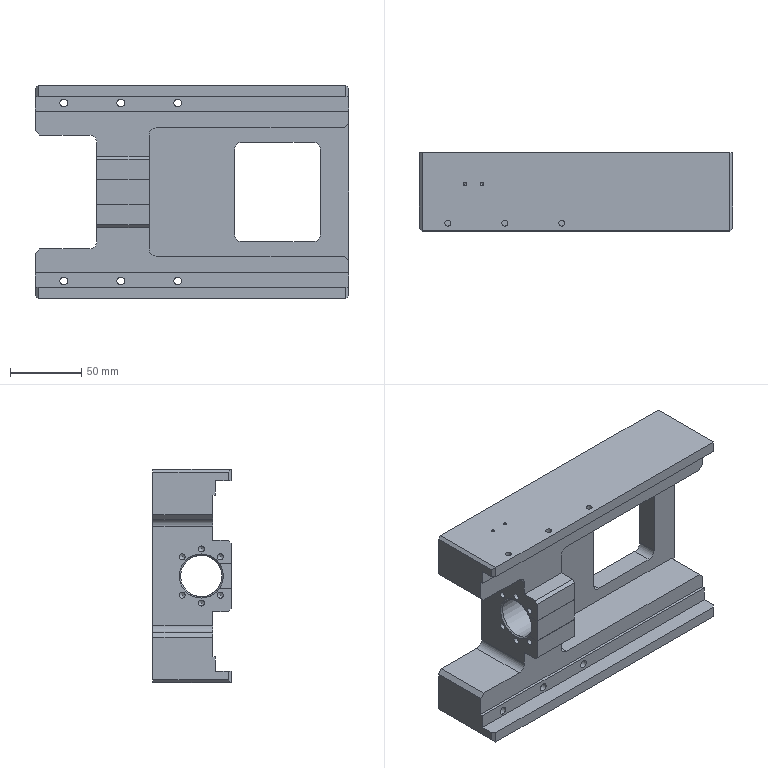CAM job | NX | 3+2 milling, drilling | part box 220 x 55 x 150 mm | stock box 225 x 60 x 155 mm
Tools:
number,name,description,diameter,corner_radius,flute_length,length,flutes
6,D6,平底铣刀-粗,6.0,0.0,25.0,75.0,2
9,D10,平底铣刀-粗,10.0,0.0,35.0,75.0,2
17,D16,平底铣刀-粗,16.0,0.0,50.0,75.0,2
7,D6-J,平底铣刀-精,6.0,0.0,25.0,75.0,2
10,D10-J,平底铣刀-精,10.0,0.0,35.0,75.0,2
18,D16-J,平底铣刀-精,16.0,0.0,50.0,75.0,2
1,D80R0.8飞刀,圆鼻刀-粗,80.0,0.8,50.0,75.0,2
1,D80R0.8飞刀-J,圆鼻刀-精,80.0,0.8,50.0,75.0,2
2,D6倒角刀,倒角刀,6.0,0.0,3.0,25.0,2
19,D10倒角刀,倒角刀,10.0,0.0,5.0,75.0,2
18,M6X1.0,丝锥,5.0,0.0,35.0,50.0,2
15,ZT5,钻头,5.0,0.0,35.0,50.0,2
17,ZT5.5,钻头,5.5,0.0,35.0,50.0,2
14,钻头4.2,Twist Drill 4.2 mm,4.2,0.0,41.0,41.738,2
Operations:
program,operation,operation_type,tool,method,geometry_group,spindle_rpm,surface_speed,feed_per_tooth,feed_cut,feed_plunge,cut_length_mm,path_length_mm,cut_time_min,machine_time_min
C,等高往复层切开粗-中_COPY,ZLevelMilling,D16,分层开粗-切深K-步距G,W-C,5000.0,251.327,0.4,4000.0,100.0,6927.946,7129.946,1.732,1.752
C,打点-深0.8_2,Operation,D10倒角刀,NONE,W-C,5000.0,157.08,0.05,500.0,90.0,10.8,237.794,0.0216,0.0443
C,盲锥孔-M5螺纹底孔,Operation,钻头4.2,NONE,W-C,2500.0,32.987,0.03,150.0,90.0,87.971,392.136,0.5865,0.6169
C,铣倒角_3,PlanarMilling,D10倒角刀,METHOD,W-C,5000.0,157.08,0.05,500.0,100.0,86.111,935.558,0.1722,0.2572
C,底壁铣倒角_COPY_1,VolumeBased25DMillingOperation,D10倒角刀,爬面_倒角-切深0-步距G,W-C,5000.0,157.08,0.05,500.0,100.0,98.589,224.989,0.1972,0.2098
C,C0.3封闭铣廓倒角6X45L_COPY,PlanarMilling,D10倒角刀,爬面_倒角-切深0-步距G,W-C,5000.0,157.08,0.15,1500.0,100.0,41.144,301.88,0.0274,0.0535
C,底壁铣精光侧面-中_COPY,VolumeBased25DMillingOperation,D16-J,侧刃精光-切深K-步距G,W-C,5000.0,251.327,0.1,1000.0,100.0,431.631,640.548,0.4316,0.4525
B,底壁铣飞面开粗_COPY,VolumeBased25DMillingOperation,D80R0.8飞刀,分层开粗-切深K-步距G,W-B,2800.0,703.696,0.5357,3000.0,100.0,8995.189,11896.094,2.998,3.288
B,底壁铣飞面精光_COPY,VolumeBased25DMillingOperation,D80R0.8飞刀-J,侧刃精光-切深K-步距G,W-B,4000.0,1005.28,0.125,1000.0,100.0,998.658,1034.658,0.9987,1.002
B,型腔铣开粗-中_COPY_1,CavityMilling,D10,分层开粗-切深K-步距G,W-B,8000.0,251.327,0.3438,5500.0,100.0,177634.57,185500.312,32.297,33.369
B,底壁铣精光底面-中_COPY,VolumeBased25DMillingOperation,D10-J,精光步距切深关,W-B,7000.0,175.0,0.0536,1500.0,100.0,3210.716,3490.119,2.14,2.168
B,底壁铣精光底面-中_COPY_1,VolumeBased25DMillingOperation,D10-J,精光步距切深关,W-B,7000.0,175.0,0.0536,1500.0,100.0,2341.522,2449.522,1.561,1.572
B,底壁铣精光侧面-中-选底面_COPY_1,VolumeBased25DMillingOperation,D10-J,侧刃精光-切深K-步距G,W-B,8000.0,251.32,0.0625,1000.0,100.0,588.723,828.896,0.5887,0.6127
B,底壁铣精光侧面-中-选底面_COPY_2,VolumeBased25DMillingOperation,D10-J,侧刃精光-切深K-步距G,W-B,8000.0,251.32,0.0625,1000.0,100.0,1114.927,1384.071,1.115,1.142
B,平面去毛刺6X45L_COPY,SurfaceContour,D6倒角刀,爬面_倒角-切深0-步距G,W-B,6500.0,122.519,0.1154,1500.0,100.0,2584.887,4812.187,1.723,1.946
B,底壁铣倒角_COPY,VolumeBased25DMillingOperation,D6倒角刀,爬面_倒角-切深0-步距G,W-B,6500.0,122.519,0.1154,1500.0,100.0,170.429,986.413,0.1136,0.1952
B,底壁铣精光侧面-中-选底面_COPY,VolumeBased25DMillingOperation,D10-J,侧刃精光-切深K-步距G,W-B,8000.0,251.32,0.0625,1000.0,100.0,476.566,671.587,0.4766,0.4961
A,顶面,FaceMilling,D80R0.8飞刀,侧刃精光-切深K-步距G,W-A,4000.0,1005.31,0.125,1000.0,100.0,1352.0,1388.0,1.352,1.356
A,型腔铣开粗-中_COPY,CavityMilling,D10,分层开粗-切深K-步距G,W-A,8000.0,251.327,0.3125,5000.0,100.0,235642.629,238423.229,47.129,47.55
A,打点-深0.8,Operation,D6倒角刀,NONE,W-A,8000.0,150.796,0.0312,500.0,90.0,21.6,582.327,0.0432,0.0993
A,盲锥孔-M6螺纹底孔,Operation,ZT5,NONE,W-A,2500.0,39.27,0.03,150.0,90.0,117.013,654.064,0.7801,0.8338
A,沉头孔-钻孔0段,Operation,ZT5.5,NONE,W-A,1200.0,20.735,0.0625,150.0,90.0,291.914,913.882,1.946,2.008
A,框开粗_1,VolumeBased25DMillingOperation,D10,METHOD,W-A,6000.0,188.0,0.25,4000.0,80.0,6577.516,6629.916,1.644,1.65
A,铣孔开粗D6_1,CylinderMilling,D6,NONE,W-A,8000.0,150.796,0.075,1200.0,100.0,3763.689,4435.689,3.136,3.204
A,铣孔精光D6_1,CylinderMilling,D6-J,精光步距切深关,W-A,8000.0,150.796,0.0312,500.0,100.0,518.489,1193.489,1.037,1.105
A,框半精_1,VolumeBased25DMillingOperation,D6-J,METHOD,W-A,6000.0,113.0,0.0833,1000.0,100.0,477.215,543.732,0.4772,0.4839
A,框精_1,VolumeBased25DMillingOperation,D6-J,METHOD,W-A,6000.0,113.0,0.0833,1000.0,100.0,238.407,305.207,0.2384,0.2451
A,仅选体,SurfaceContour,D6倒角刀,METHOD,W-A,8000.0,150.796,0.1875,3000.0,100.0,1083.197,1238.677,0.3611,0.3766
A,铣倒角_1,PlanarMilling,D6倒角刀,METHOD,W-A,8000.0,150.796,0.0375,600.0,100.0,113.732,738.343,0.1896,0.252
A,铣倒角_2,PlanarMilling,D6倒角刀,NONE,W-A,8000.0,150.796,0.05,800.0,100.0,241.506,738.047,0.3019,0.3515
A,盲锥孔-攻牙M6,Operation,M6X1.0,METHOD,W-A,500.0,7.854,0.001,1.0,90.0,96.0,612.038,96.0,96.052
A,外形半精_2,VolumeBased25DMillingOperation,D10-J,METHOD,W-A,8000.0,251.327,0.0625,1000.0,100.0,2549.643,2891.672,2.55,2.584